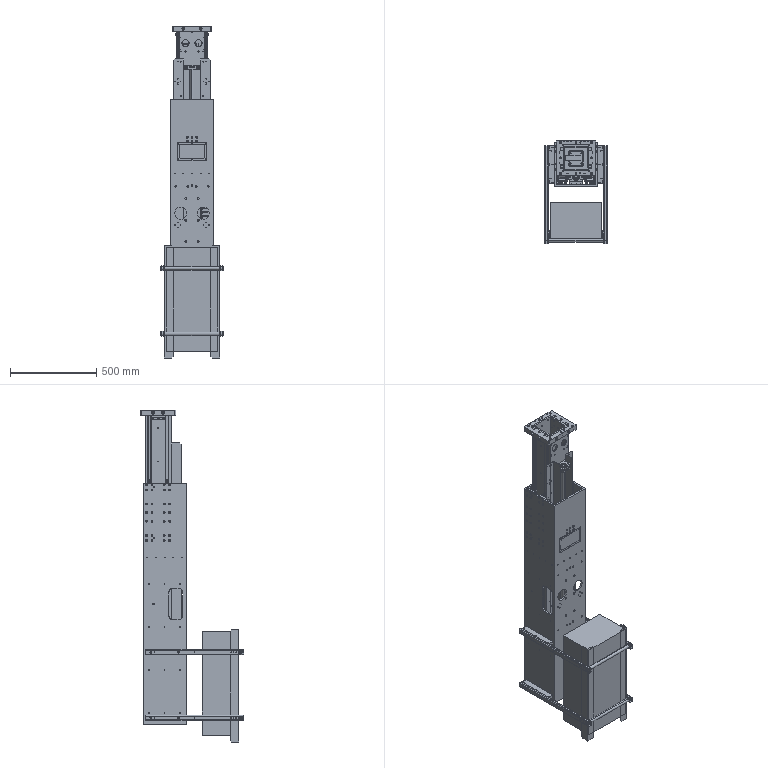Part | SolidWorks | features InContextFeatHolder 16 | 238 solids | 19852 faces | volume 69065050 mm3 | plane 10226 | cylinder 8087 | cone 1059 | spline 328 | sphere 96 | torus 56 | commonest cylinder face diameters 1 x1690 10 x738 0.2 x544 2 x444 5 x426 20 x355